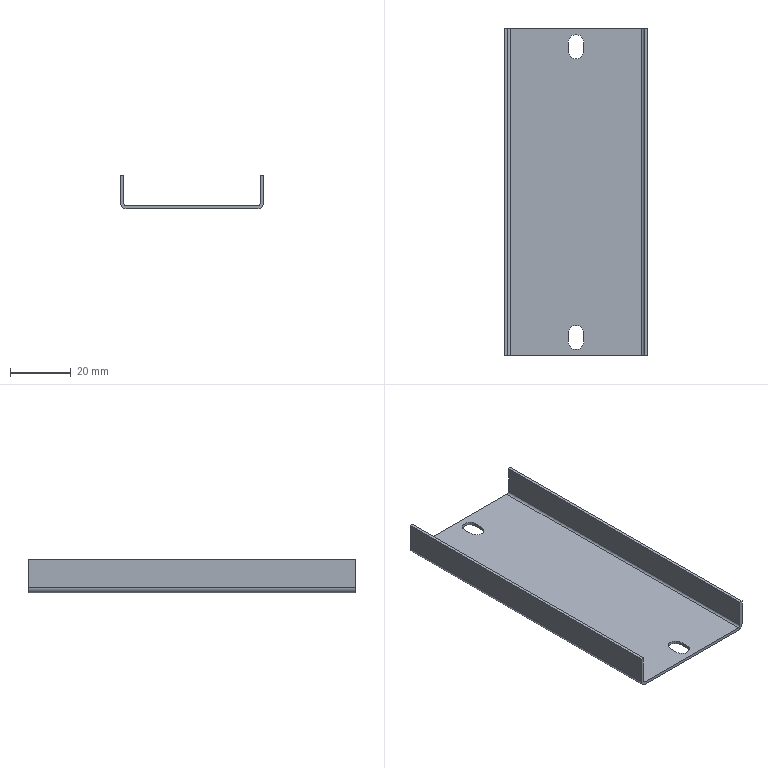Part | STEP file | door handle rear cover (SUS304) | 1 solid | 22 faces | box 47 x 108 x 11 mm | volume 7052 mm3 | plane 14 | cylinder 8 | commonest cylinder face diameters 5 x4 1.473 x2 3.473 x2